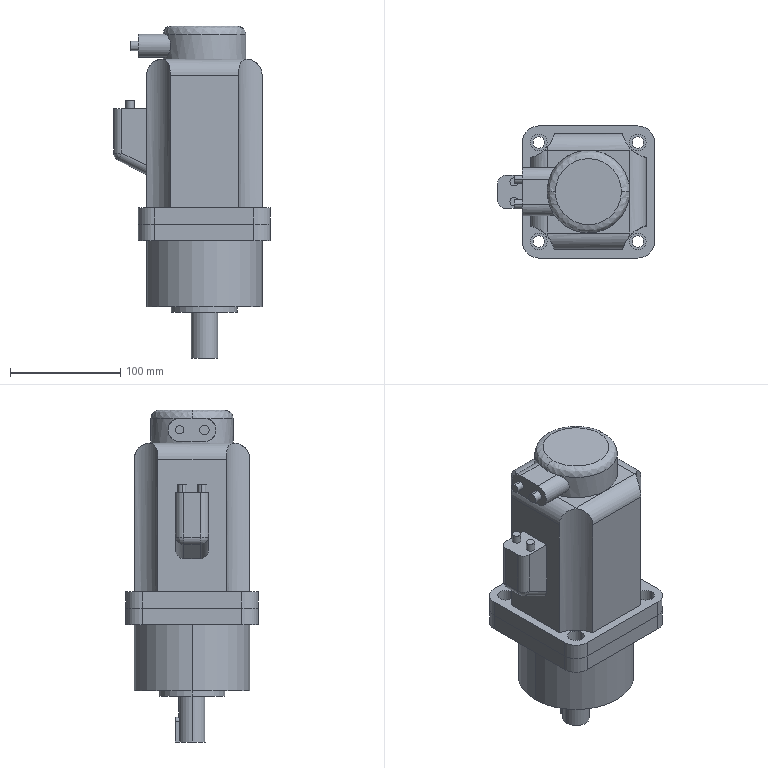Part | SolidWorks | features ICE 3, BaseBody 2, 3DProfileFeature 1, HoleWzd 1 | 2 solids | 127 faces | box 142.5 x 120 x 301.5 mm | volume 2581853 mm3 | cylinder 71 | plane 46 | spline 8 | cone 2 | commonest cylinder face diameters 7.5 x20 15 x13 30 x12 10.5 x8 60 x6 5 x2